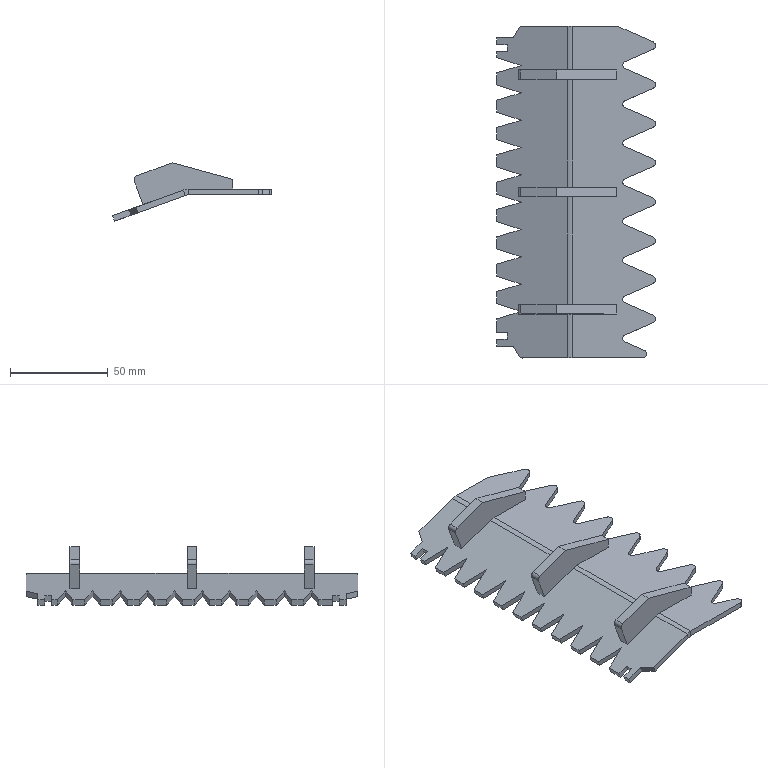Part | SolidWorks | features BaseBody 1, ICE 1, MirrorSolid 1 | 1 solid | 113 faces | box 81.389 x 170 x 29.968 mm | volume 44685 mm3 | plane 88 | cylinder 25 | commonest cylinder face diameters 4 x20 16 x4 10 x1